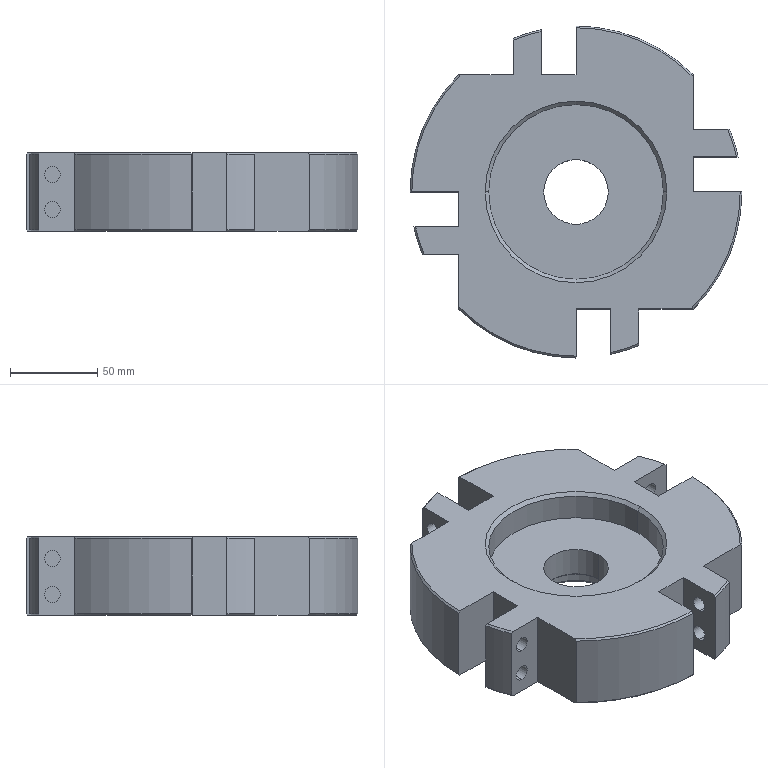Part | SolidWorks | features 3DProfileFeature 5, Chamfer 5, HoleWzd 5, ICE 2, Extrusion 1 | 1 solid | 76 faces | box 190 x 190 x 45 mm | volume 928420 mm3 | cylinder 30 | plane 24 | cone 22 | commonest cylinder face diameters 9 x16 190 x8 37 x2 49.5 x2 100 x2